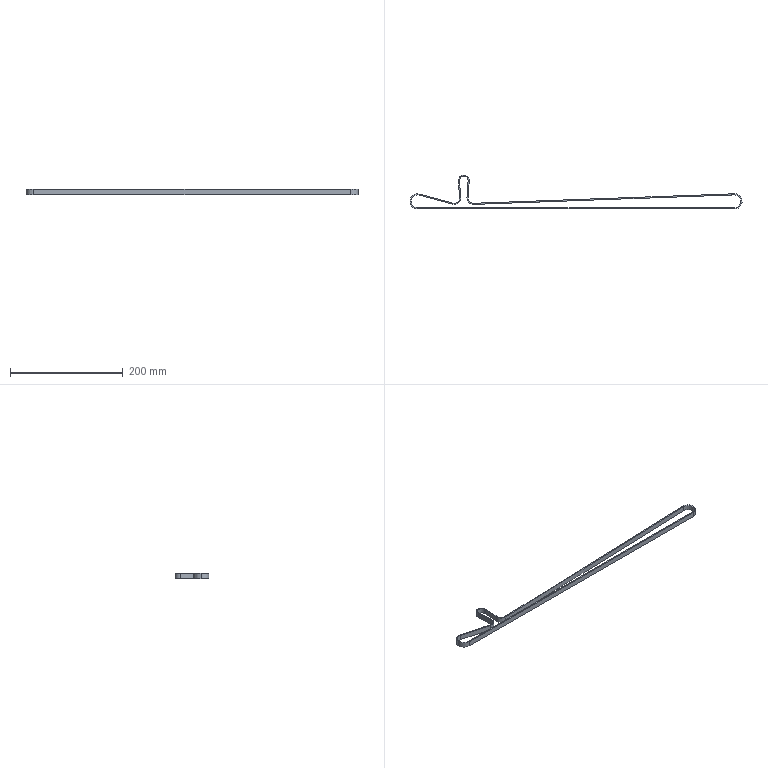Part | STEP file | Timing belt 1293-3M-9mm wide | 1 solid | 30 faces | box 588.86 x 60.04 x 9 mm | volume 23269 mm3 | cylinder 18 | plane 12 | commonest cylinder face diameters 15.22 x3 18.94 x3 19.22 x3 22.86 x3 22.94 x3 26.86 x3